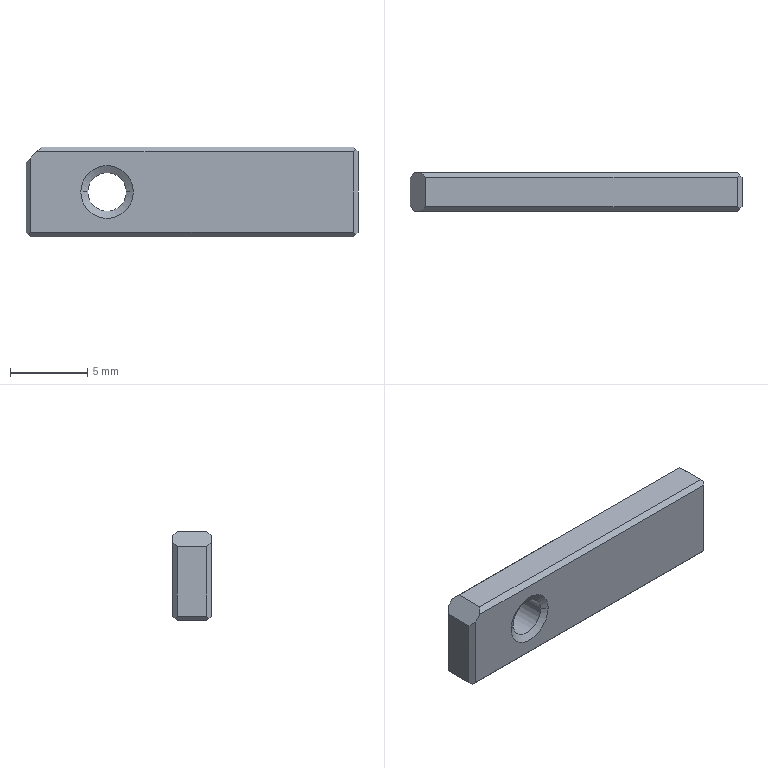Part | NX | 1 solid | 22 faces | box 21.5 x 2.5 x 5.8 mm | volume 292.746 mm3 | plane 18 | cylinder 2 | cone 2 | commonest cylinder face diameters 2.5 x2
STEP:
#1=CARTESIAN_POINT('',(-222.5,223.3,-37.742));
#2=VERTEX_POINT('',#1);
#3=CARTESIAN_POINT('',(-222.5,225.2,-37.742));
#4=VERTEX_POINT('',#3);
#5=CARTESIAN_POINT('',(-222.5,224.25,-37.742));
#6=DIRECTION('',(0.,1.,0.));
#7=VECTOR('',#6,1000.);
#8=LINE('',#5,#7);
#9=EDGE_CURVE('',#2,#4,#8,.T.);
#10=ORIENTED_EDGE('',*,*,#9,.F.);
#11=CARTESIAN_POINT('',(-202.3,223.3,-37.742));
#12=VERTEX_POINT('',#11);
#13=CARTESIAN_POINT('',(-212.75,223.3,-37.742));
#14=DIRECTION('',(-1.,0.,0.));
#15=VECTOR('',#14,1000.);
#16=LINE('',#13,#15);
#17=EDGE_CURVE('',#12,#2,#16,.T.);
#18=ORIENTED_EDGE('',*,*,#17,.F.);
#19=CARTESIAN_POINT('',(-202.3,225.2,-37.742));
#20=VERTEX_POINT('',#19);
#21=CARTESIAN_POINT('',(-202.3,224.25,-37.742));
#22=DIRECTION('',(0.,1.,0.));
#23=VECTOR('',#22,1000.);
#24=LINE('',#21,#23);
#25=EDGE_CURVE('',#12,#20,#24,.T.);
#26=ORIENTED_EDGE('',*,*,#25,.T.);
#27=CARTESIAN_POINT('',(-212.75,225.2,-37.742));
#28=DIRECTION('',(-1.,0.,0.));
#29=VECTOR('',#28,1000.);
#30=LINE('',#27,#29);
#31=EDGE_CURVE('',#20,#4,#30,.T.);
#32=ORIENTED_EDGE('',*,*,#31,.T.);
#33=EDGE_LOOP('',(#10,#18,#26,#32));
#34=FACE_BOUND('',#33,.T.);
#35=CARTESIAN_POINT('',(-213.,223.,-37.742));
#36=DIRECTION('',(0.,0.,1.));
#37=DIRECTION('',(0.,-1.,0.));
#38=AXIS2_PLACEMENT_3D('',#35,#36,#37);
#39=PLANE('',#38);
#40=ADVANCED_FACE('',(#34),#39,.T.);
#41=CARTESIAN_POINT('',(-223.5,223.3,-38.742));
#42=VERTEX_POINT('',#41);
#43=CARTESIAN_POINT('',(-223.5,223.3,-43.242));
#44=VERTEX_POINT('',#43);
#45=CARTESIAN_POINT('',(-223.5,223.3,-40.642));
#46=DIRECTION('',(0.,0.,-1.));
#47=VECTOR('',#46,1000.);
#48=LINE('',#45,#47);
#49=EDGE_CURVE('',#42,#44,#48,.T.);
#50=ORIENTED_EDGE('',*,*,#49,.F.);
#51=CARTESIAN_POINT('',(-223.5,225.2,-38.742));
#52=VERTEX_POINT('',#51);
#53=CARTESIAN_POINT('',(-223.5,224.25,-38.742));
#54=DIRECTION('',(0.,1.,0.));
#55=VECTOR('',#54,1000.);
#56=LINE('',#53,#55);
#57=EDGE_CURVE('',#42,#52,#56,.T.);
#58=ORIENTED_EDGE('',*,*,#57,.T.);
#59=CARTESIAN_POINT('',(-223.5,225.2,-43.242));
#60=VERTEX_POINT('',#59);
#61=CARTESIAN_POINT('',(-223.5,225.2,-40.642));
#62=DIRECTION('',(0.,0.,-1.));
#63=VECTOR('',#62,1000.);
#64=LINE('',#61,#63);
#65=EDGE_CURVE('',#52,#60,#64,.T.);
#66=ORIENTED_EDGE('',*,*,#65,.T.);
#67=CARTESIAN_POINT('',(-223.5,224.25,-43.242));
#68=DIRECTION('',(0.,1.,0.));
#69=VECTOR('',#68,1000.);
#70=LINE('',#67,#69);
#71=EDGE_CURVE('',#44,#60,#70,.T.);
#72=ORIENTED_EDGE('',*,*,#71,.F.);
#73=EDGE_LOOP('',(#50,#58,#66,#72));
#74=FACE_BOUND('',#73,.T.);
#75=CARTESIAN_POINT('',(-223.5,223.,-37.742));
#76=DIRECTION('',(-1.,0.,0.));
#77=DIRECTION('',(0.,1.,0.));
#78=AXIS2_PLACEMENT_3D('',#75,#76,#77);
#79=PLANE('',#78);
#80=ADVANCED_FACE('',(#74),#79,.T.);
#81=CARTESIAN_POINT('',(-223.2,223.3,-43.542));
#82=VERTEX_POINT('',#81);
#83=CARTESIAN_POINT('',(-223.2,225.2,-43.542));
#84=VERTEX_POINT('',#83);
#85=CARTESIAN_POINT('',(-223.2,224.25,-43.542));
#86=DIRECTION('',(0.,1.,0.));
#87=VECTOR('',#86,1000.);
#88=LINE('',#85,#87);
#89=EDGE_CURVE('',#82,#84,#88,.T.);
#90=ORIENTED_EDGE('',*,*,#89,.T.);
#91=CARTESIAN_POINT('',(-202.3,225.2,-43.542));
#92=VERTEX_POINT('',#91);
#93=CARTESIAN_POINT('',(-212.75,225.2,-43.542));
#94=DIRECTION('',(1.,0.,0.));
#95=VECTOR('',#94,1000.);
#96=LINE('',#93,#95);
#97=EDGE_CURVE('',#84,#92,#96,.T.);
#98=ORIENTED_EDGE('',*,*,#97,.T.);
#99=CARTESIAN_POINT('',(-202.3,223.3,-43.542));
#100=VERTEX_POINT('',#99);
#101=CARTESIAN_POINT('',(-202.3,224.25,-43.542));
#102=DIRECTION('',(0.,1.,0.));
#103=VECTOR('',#102,1000.);
#104=LINE('',#101,#103);
#105=EDGE_CURVE('',#100,#92,#104,.T.);
#106=ORIENTED_EDGE('',*,*,#105,.F.);
#107=CARTESIAN_POINT('',(-212.75,223.3,-43.542));
#108=DIRECTION('',(1.,0.,0.));
#109=VECTOR('',#108,1000.);
#110=LINE('',#107,#109);
#111=EDGE_CURVE('',#82,#100,#110,.T.);
#112=ORIENTED_EDGE('',*,*,#111,.F.);
#113=EDGE_LOOP('',(#90,#98,#106,#112));
#114=FACE_BOUND('',#113,.T.);
#115=CARTESIAN_POINT('',(-223.5,223.,-43.542));
#116=DIRECTION('',(0.,0.,-1.));
#117=DIRECTION('',(-1.,0.,0.));
#118=AXIS2_PLACEMENT_3D('',#115,#116,#117);
#119=PLANE('',#118);
#120=ADVANCED_FACE('',(#114),#119,.T.);
#121=CARTESIAN_POINT('',(-217.,223.26,-40.642));
#122=VERTEX_POINT('',#121);
#123=CARTESIAN_POINT('',(-219.5,223.26,-40.642));
#124=VERTEX_POINT('',#123);
#125=CARTESIAN_POINT('',(-218.25,223.26,-40.642));
#126=DIRECTION('',(0.,-1.,0.));
#127=DIRECTION('',(-1.,0.,0.));
#128=AXIS2_PLACEMENT_3D('',#125,#126,#127);
#129=CIRCLE('',#128,1.25);
#130=EDGE_CURVE('',#122,#124,#129,.T.);
#131=ORIENTED_EDGE('',*,*,#130,.T.);
#132=CARTESIAN_POINT('',(-219.5,225.5,-40.642));
#133=VERTEX_POINT('',#132);
#134=CARTESIAN_POINT('',(-219.5,223.,-40.642));
#135=DIRECTION('',(0.,-1.,0.));
#136=VECTOR('',#135,1000.);
#137=LINE('',#134,#136);
#138=EDGE_CURVE('',#124,#133,#137,.F.);
#139=ORIENTED_EDGE('',*,*,#138,.T.);
#140=CARTESIAN_POINT('',(-217.,225.5,-40.642));
#141=VERTEX_POINT('',#140);
#142=CARTESIAN_POINT('',(-218.25,225.5,-40.642));
#143=DIRECTION('',(0.,-1.,0.));
#144=DIRECTION('',(-1.,0.,0.));
#145=AXIS2_PLACEMENT_3D('',#142,#143,#144);
#146=CIRCLE('',#145,1.25);
#147=EDGE_CURVE('',#141,#133,#146,.T.);
#148=ORIENTED_EDGE('',*,*,#147,.F.);
#149=CARTESIAN_POINT('',(-217.,223.,-40.642));
#150=DIRECTION('',(0.,-1.,0.));
#151=VECTOR('',#150,1000.);
#152=LINE('',#149,#151);
#153=EDGE_CURVE('',#122,#141,#152,.F.);
#154=ORIENTED_EDGE('',*,*,#153,.F.);
#155=EDGE_LOOP('',(#131,#139,#148,#154));
#156=FACE_BOUND('',#155,.T.);
#157=CARTESIAN_POINT('',(-218.25,223.,-40.642));
#158=DIRECTION('',(0.,-1.,0.));
#159=DIRECTION('',(-1.,0.,0.));
#160=AXIS2_PLACEMENT_3D('',#157,#158,#159);
#161=CYLINDRICAL_SURFACE('',#160,1.25);
#162=ADVANCED_FACE('',(#156),#161,.F.);
#163=ORIENTED_EDGE('',*,*,#130,.F.);
#164=CARTESIAN_POINT('',(-216.55,223.,-40.642));
#165=VERTEX_POINT('',#164);
#166=CARTESIAN_POINT('',(-217.,223.26,-40.642));
#167=DIRECTION('',(0.866,-0.5,0.));
#168=VECTOR('',#167,1000.);
#169=LINE('',#166,#168);
#170=EDGE_CURVE('',#165,#122,#169,.F.);
#171=ORIENTED_EDGE('',*,*,#170,.F.);
#172=CARTESIAN_POINT('',(-219.95,223.,-40.642));
#173=VERTEX_POINT('',#172);
#174=CARTESIAN_POINT('',(-218.25,223.,-40.642));
#175=DIRECTION('',(0.,-1.,0.));
#176=DIRECTION('',(-1.,0.,0.));
#177=AXIS2_PLACEMENT_3D('',#174,#175,#176);
#178=CIRCLE('',#177,1.7);
#179=EDGE_CURVE('',#165,#173,#178,.T.);
#180=ORIENTED_EDGE('',*,*,#179,.T.);
#181=CARTESIAN_POINT('',(-219.5,223.26,-40.642));
#182=DIRECTION('',(-0.866,-0.5,0.));
#183=VECTOR('',#182,1000.);
#184=LINE('',#181,#183);
#185=EDGE_CURVE('',#173,#124,#184,.F.);
#186=ORIENTED_EDGE('',*,*,#185,.T.);
#187=EDGE_LOOP('',(#163,#171,#180,#186));
#188=FACE_BOUND('',#187,.T.);
#189=CARTESIAN_POINT('',(-218.25,223.26,-40.642));
#190=DIRECTION('',(0.,-1.,0.));
#191=DIRECTION('',(-1.,0.,0.));
#192=AXIS2_PLACEMENT_3D('',#189,#190,#191);
#193=CONICAL_SURFACE('',#192,1.25,1.047);
#194=ADVANCED_FACE('',(#188),#193,.F.);
#195=ORIENTED_EDGE('',*,*,#97,.F.);
#196=CARTESIAN_POINT('',(-223.35,225.35,-43.392));
#197=VERTEX_POINT('',#196);
#198=CARTESIAN_POINT('',(-221.,223.,-45.742));
#199=DIRECTION('',(-0.5774,0.5774,0.5774));
#200=VECTOR('',#199,1000.);
#201=LINE('',#198,#200);
#202=EDGE_CURVE('',#84,#197,#201,.T.);
#203=ORIENTED_EDGE('',*,*,#202,.T.);
#204=CARTESIAN_POINT('',(-223.2,225.5,-43.242));
#205=VERTEX_POINT('',#204);
#206=CARTESIAN_POINT('',(-225.7,223.,-45.742));
#207=DIRECTION('',(-0.5774,-0.5774,-0.5774));
#208=VECTOR('',#207,1000.);
#209=LINE('',#206,#208);
#210=EDGE_CURVE('',#205,#197,#209,.T.);
#211=ORIENTED_EDGE('',*,*,#210,.F.);
#212=CARTESIAN_POINT('',(-202.3,225.5,-43.242));
#213=VERTEX_POINT('',#212);
#214=CARTESIAN_POINT('',(-212.75,225.5,-43.242));
#215=DIRECTION('',(1.,0.,0.));
#216=VECTOR('',#215,1000.);
#217=LINE('',#214,#216);
#218=EDGE_CURVE('',#205,#213,#217,.T.);
#219=ORIENTED_EDGE('',*,*,#218,.T.);
#220=CARTESIAN_POINT('',(-202.15,225.35,-43.392));
#221=VERTEX_POINT('',#220);
#222=CARTESIAN_POINT('',(-218.25,241.45,-27.292));
#223=DIRECTION('',(-0.5774,0.5774,0.5774));
#224=VECTOR('',#223,1000.);
#225=LINE('',#222,#224);
#226=EDGE_CURVE('',#221,#213,#225,.T.);
#227=ORIENTED_EDGE('',*,*,#226,.F.);
#228=CARTESIAN_POINT('',(-218.25,209.25,-59.492));
#229=DIRECTION('',(0.5774,0.5774,0.5774));
#230=VECTOR('',#229,1000.);
#231=LINE('',#228,#230);
#232=EDGE_CURVE('',#92,#221,#231,.T.);
#233=ORIENTED_EDGE('',*,*,#232,.F.);
#234=EDGE_LOOP('',(#195,#203,#211,#219,#227,#233));
#235=FACE_BOUND('',#234,.T.);
#236=CARTESIAN_POINT('',(-212.75,225.35,-43.392));
#237=DIRECTION('',(0.,0.7071,-0.7071));
#238=DIRECTION('',(-1.,0.,0.));
#239=AXIS2_PLACEMENT_3D('',#236,#237,#238);
#240=PLANE('',#239);
#241=ADVANCED_FACE('',(#235),#240,.T.);
#242=ORIENTED_EDGE('',*,*,#89,.F.);
#243=CARTESIAN_POINT('',(-223.35,223.15,-43.392));
#244=VERTEX_POINT('',#243);
#245=CARTESIAN_POINT('',(-223.5,223.,-43.242));
#246=DIRECTION('',(0.5774,0.5774,-0.5774));
#247=VECTOR('',#246,1000.);
#248=LINE('',#245,#247);
#249=EDGE_CURVE('',#244,#82,#248,.T.);
#250=ORIENTED_EDGE('',*,*,#249,.F.);
#251=CARTESIAN_POINT('',(-226.1,225.9,-40.642));
#252=DIRECTION('',(-0.5774,0.5774,0.5774));
#253=VECTOR('',#252,1000.);
#254=LINE('',#251,#253);
#255=EDGE_CURVE('',#244,#44,#254,.T.);
#256=ORIENTED_EDGE('',*,*,#255,.T.);
#257=ORIENTED_EDGE('',*,*,#71,.T.);
#258=CARTESIAN_POINT('',(-226.1,222.6,-40.642));
#259=DIRECTION('',(-0.5774,-0.5774,0.5774));
#260=VECTOR('',#259,1000.);
#261=LINE('',#258,#260);
#262=EDGE_CURVE('',#197,#60,#261,.T.);
#263=ORIENTED_EDGE('',*,*,#262,.F.);
#264=ORIENTED_EDGE('',*,*,#202,.F.);
#265=EDGE_LOOP('',(#242,#250,#256,#257,#263,#264));
#266=FACE_BOUND('',#265,.T.);
#267=CARTESIAN_POINT('',(-223.35,224.25,-43.392));
#268=DIRECTION('',(-0.7071,0.,-0.7071));
#269=DIRECTION('',(-0.7071,0.,0.7071));
#270=AXIS2_PLACEMENT_3D('',#267,#268,#269);
#271=PLANE('',#270);
#272=ADVANCED_FACE('',(#266),#271,.T.);
#273=ORIENTED_EDGE('',*,*,#9,.T.);
#274=CARTESIAN_POINT('',(-222.8,225.5,-38.042));
#275=VERTEX_POINT('',#274);
#276=CARTESIAN_POINT('',(-220.3,223.,-35.542));
#277=DIRECTION('',(-0.5774,0.5774,-0.5774));
#278=VECTOR('',#277,1000.);
#279=LINE('',#276,#278);
#280=EDGE_CURVE('',#4,#275,#279,.T.);
#281=ORIENTED_EDGE('',*,*,#280,.T.);
#282=CARTESIAN_POINT('',(-223.2,225.5,-38.442));
#283=VERTEX_POINT('',#282);
#284=CARTESIAN_POINT('',(-225.4,225.5,-40.642));
#285=DIRECTION('',(0.7071,0.,0.7071));
#286=VECTOR('',#285,1000.);
#287=LINE('',#284,#286);
#288=EDGE_CURVE('',#283,#275,#287,.T.);
#289=ORIENTED_EDGE('',*,*,#288,.F.);
#290=CARTESIAN_POINT('',(-225.7,223.,-40.942));
#291=DIRECTION('',(-0.5774,-0.5774,-0.5774));
#292=VECTOR('',#291,1000.);
#293=LINE('',#290,#292);
#294=EDGE_CURVE('',#283,#52,#293,.T.);
#295=ORIENTED_EDGE('',*,*,#294,.T.);
#296=ORIENTED_EDGE('',*,*,#57,.F.);
#297=CARTESIAN_POINT('',(-223.2,223.,-38.442));
#298=VERTEX_POINT('',#297);
#299=CARTESIAN_POINT('',(-223.2,223.,-38.442));
#300=DIRECTION('',(-0.5774,0.5774,-0.5774));
#301=VECTOR('',#300,1000.);
#302=LINE('',#299,#301);
#303=EDGE_CURVE('',#298,#42,#302,.T.);
#304=ORIENTED_EDGE('',*,*,#303,.F.);
#305=CARTESIAN_POINT('',(-222.8,223.,-38.042));
#306=VERTEX_POINT('',#305);
#307=CARTESIAN_POINT('',(-225.4,223.,-40.642));
#308=DIRECTION('',(0.7071,0.,0.7071));
#309=VECTOR('',#308,1000.);
#310=LINE('',#307,#309);
#311=EDGE_CURVE('',#298,#306,#310,.T.);
#312=ORIENTED_EDGE('',*,*,#311,.T.);
#313=CARTESIAN_POINT('',(-222.8,223.,-38.042));
#314=DIRECTION('',(-0.5774,-0.5774,-0.5774));
#315=VECTOR('',#314,1000.);
#316=LINE('',#313,#315);
#317=EDGE_CURVE('',#2,#306,#316,.T.);
#318=ORIENTED_EDGE('',*,*,#317,.F.);
#319=EDGE_LOOP('',(#273,#281,#289,#295,#296,#304,#312,#318));
#320=FACE_BOUND('',#319,.T.);
#321=CARTESIAN_POINT('',(-223.,224.25,-38.242));
#322=DIRECTION('',(0.7071,0.,-0.7071));
#323=DIRECTION('',(0.,-1.,0.));
#324=AXIS2_PLACEMENT_3D('',#321,#322,#323);
#325=PLANE('',#324);
#326=ADVANCED_FACE('',(#320),#325,.F.);
#327=ORIENTED_EDGE('',*,*,#138,.F.);
#328=CARTESIAN_POINT('',(-218.25,223.26,-40.642));
#329=DIRECTION('',(0.,-1.,0.));
#330=DIRECTION('',(-1.,0.,0.));
#331=AXIS2_PLACEMENT_3D('',#328,#329,#330);
#332=CIRCLE('',#331,1.25);
#333=EDGE_CURVE('',#124,#122,#332,.T.);
#334=ORIENTED_EDGE('',*,*,#333,.T.);
#335=ORIENTED_EDGE('',*,*,#153,.T.);
#336=CARTESIAN_POINT('',(-218.25,225.5,-40.642));
#337=DIRECTION('',(0.,-1.,0.));
#338=DIRECTION('',(-1.,0.,0.));
#339=AXIS2_PLACEMENT_3D('',#336,#337,#338);
#340=CIRCLE('',#339,1.25);
#341=EDGE_CURVE('',#133,#141,#340,.T.);
#342=ORIENTED_EDGE('',*,*,#341,.F.);
#343=EDGE_LOOP('',(#327,#334,#335,#342));
#344=FACE_BOUND('',#343,.T.);
#345=CARTESIAN_POINT('',(-218.25,223.,-40.642));
#346=DIRECTION('',(0.,-1.,0.));
#347=DIRECTION('',(-1.,0.,0.));
#348=AXIS2_PLACEMENT_3D('',#345,#346,#347);
#349=CYLINDRICAL_SURFACE('',#348,1.25);
#350=ADVANCED_FACE('',(#344),#349,.F.);
#351=ORIENTED_EDGE('',*,*,#185,.F.);
#352=CARTESIAN_POINT('',(-218.25,223.,-40.642));
#353=DIRECTION('',(0.,-1.,0.));
#354=DIRECTION('',(-1.,0.,0.));
#355=AXIS2_PLACEMENT_3D('',#352,#353,#354);
#356=CIRCLE('',#355,1.7);
#357=EDGE_CURVE('',#173,#165,#356,.T.);
#358=ORIENTED_EDGE('',*,*,#357,.T.);
#359=ORIENTED_EDGE('',*,*,#170,.T.);
#360=ORIENTED_EDGE('',*,*,#333,.F.);
#361=EDGE_LOOP('',(#351,#358,#359,#360));
#362=FACE_BOUND('',#361,.T.);
#363=CARTESIAN_POINT('',(-218.25,223.26,-40.642));
#364=DIRECTION('',(0.,-1.,0.));
#365=DIRECTION('',(-1.,0.,0.));
#366=AXIS2_PLACEMENT_3D('',#363,#364,#365);
#367=CONICAL_SURFACE('',#366,1.25,1.047);
#368=ADVANCED_FACE('',(#362),#367,.F.);
#369=CARTESIAN_POINT('',(-223.2,225.5,-40.642));
#370=DIRECTION('',(0.,0.,-1.));
#371=VECTOR('',#370,1000.);
#372=LINE('',#369,#371);
#373=EDGE_CURVE('',#283,#205,#372,.T.);
#374=ORIENTED_EDGE('',*,*,#373,.F.);
#375=ORIENTED_EDGE('',*,*,#288,.T.);
#376=CARTESIAN_POINT('',(-202.3,225.5,-38.042));
#377=VERTEX_POINT('',#376);
#378=CARTESIAN_POINT('',(-212.75,225.5,-38.042));
#379=DIRECTION('',(-1.,0.,0.));
#380=VECTOR('',#379,1000.);
#381=LINE('',#378,#380);
#382=EDGE_CURVE('',#377,#275,#381,.T.);
#383=ORIENTED_EDGE('',*,*,#382,.F.);
#384=CARTESIAN_POINT('',(-202.3,225.5,-40.642));
#385=DIRECTION('',(0.,0.,1.));
#386=VECTOR('',#385,1000.);
#387=LINE('',#384,#386);
#388=EDGE_CURVE('',#213,#377,#387,.T.);
#389=ORIENTED_EDGE('',*,*,#388,.F.);
#390=ORIENTED_EDGE('',*,*,#218,.F.);
#391=EDGE_LOOP('',(#374,#375,#383,#389,#390));
#392=FACE_BOUND('',#391,.T.);
#393=ORIENTED_EDGE('',*,*,#147,.T.);
#394=ORIENTED_EDGE('',*,*,#341,.T.);
#395=EDGE_LOOP('',(#393,#394));
#396=FACE_BOUND('',#395,.T.);
#397=CARTESIAN_POINT('',(-218.25,225.5,-40.642));
#398=DIRECTION('',(0.,1.,0.));
#399=DIRECTION('',(0.,0.,-1.));
#400=AXIS2_PLACEMENT_3D('',#397,#398,#399);
#401=PLANE('',#400);
#402=ADVANCED_FACE('',(#392,#396),#401,.T.);
#403=ORIENTED_EDGE('',*,*,#382,.T.);
#404=ORIENTED_EDGE('',*,*,#280,.F.);
#405=ORIENTED_EDGE('',*,*,#31,.F.);
#406=CARTESIAN_POINT('',(-202.15,225.35,-37.892));
#407=VERTEX_POINT('',#406);
#408=CARTESIAN_POINT('',(-218.25,209.25,-21.792));
#409=DIRECTION('',(0.5774,0.5774,-0.5774));
#410=VECTOR('',#409,1000.);
#411=LINE('',#408,#410);
#412=EDGE_CURVE('',#20,#407,#411,.T.);
#413=ORIENTED_EDGE('',*,*,#412,.T.);
#414=CARTESIAN_POINT('',(-218.25,241.45,-53.992));
#415=DIRECTION('',(-0.5774,0.5774,-0.5774));
#416=VECTOR('',#415,1000.);
#417=LINE('',#414,#416);
#418=EDGE_CURVE('',#407,#377,#417,.T.);
#419=ORIENTED_EDGE('',*,*,#418,.T.);
#420=EDGE_LOOP('',(#403,#404,#405,#413,#419));
#421=FACE_BOUND('',#420,.T.);
#422=CARTESIAN_POINT('',(-212.75,225.35,-37.892));
#423=DIRECTION('',(0.,-0.7071,-0.7071));
#424=DIRECTION('',(0.,-0.7071,0.7071));
#425=AXIS2_PLACEMENT_3D('',#422,#423,#424);
#426=PLANE('',#425);
#427=ADVANCED_FACE('',(#421),#426,.F.);
#428=ORIENTED_EDGE('',*,*,#373,.T.);
#429=ORIENTED_EDGE('',*,*,#210,.T.);
#430=ORIENTED_EDGE('',*,*,#262,.T.);
#431=ORIENTED_EDGE('',*,*,#65,.F.);
#432=ORIENTED_EDGE('',*,*,#294,.F.);
#433=EDGE_LOOP('',(#428,#429,#430,#431,#432));
#434=FACE_BOUND('',#433,.T.);
#435=CARTESIAN_POINT('',(-223.35,225.35,-40.642));
#436=DIRECTION('',(0.7071,-0.7071,0.));
#437=DIRECTION('',(0.,0.,-1.));
#438=AXIS2_PLACEMENT_3D('',#435,#436,#437);
#439=PLANE('',#438);
#440=ADVANCED_FACE('',(#434),#439,.F.);
#441=CARTESIAN_POINT('',(-202.,223.3,-43.242));
#442=VERTEX_POINT('',#441);
#443=CARTESIAN_POINT('',(-202.,225.2,-43.242));
#444=VERTEX_POINT('',#443);
#445=CARTESIAN_POINT('',(-202.,224.25,-43.242));
#446=DIRECTION('',(0.,1.,0.));
#447=VECTOR('',#446,1000.);
#448=LINE('',#445,#447);
#449=EDGE_CURVE('',#442,#444,#448,.T.);
#450=ORIENTED_EDGE('',*,*,#449,.T.);
#451=CARTESIAN_POINT('',(-202.,225.2,-38.042));
#452=VERTEX_POINT('',#451);
#453=CARTESIAN_POINT('',(-202.,225.2,-40.642));
#454=DIRECTION('',(0.,0.,1.));
#455=VECTOR('',#454,1000.);
#456=LINE('',#453,#455);
#457=EDGE_CURVE('',#444,#452,#456,.T.);
#458=ORIENTED_EDGE('',*,*,#457,.T.);
#459=CARTESIAN_POINT('',(-202.,223.3,-38.042));
#460=VERTEX_POINT('',#459);
#461=CARTESIAN_POINT('',(-202.,224.25,-38.042));
#462=DIRECTION('',(0.,1.,0.));
#463=VECTOR('',#462,1000.);
#464=LINE('',#461,#463);
#465=EDGE_CURVE('',#460,#452,#464,.T.);
#466=ORIENTED_EDGE('',*,*,#465,.F.);
#467=CARTESIAN_POINT('',(-202.,223.3,-40.642));
#468=DIRECTION('',(0.,0.,1.));
#469=VECTOR('',#468,1000.);
#470=LINE('',#467,#469);
#471=EDGE_CURVE('',#442,#460,#470,.T.);
#472=ORIENTED_EDGE('',*,*,#471,.F.);
#473=EDGE_LOOP('',(#450,#458,#466,#472));
#474=FACE_BOUND('',#473,.T.);
#475=CARTESIAN_POINT('',(-202.,223.,-43.542));
#476=DIRECTION('',(1.,0.,0.));
#477=DIRECTION('',(0.,1.,0.));
#478=AXIS2_PLACEMENT_3D('',#475,#476,#477);
#479=PLANE('',#478);
#480=ADVANCED_FACE('',(#474),#479,.T.);
#481=ORIENTED_EDGE('',*,*,#457,.F.);
#482=CARTESIAN_POINT('',(-218.25,241.45,-59.492));
#483=DIRECTION('',(-0.5774,0.5774,-0.5774));
#484=VECTOR('',#483,1000.);
#485=LINE('',#482,#484);
#486=EDGE_CURVE('',#444,#221,#485,.T.);
#487=ORIENTED_EDGE('',*,*,#486,.T.);
#488=ORIENTED_EDGE('',*,*,#226,.T.);
#489=ORIENTED_EDGE('',*,*,#388,.T.);
#490=ORIENTED_EDGE('',*,*,#418,.F.);
#491=CARTESIAN_POINT('',(-218.25,241.45,-21.792));
#492=DIRECTION('',(-0.5774,0.5774,0.5774));
#493=VECTOR('',#492,1000.);
#494=LINE('',#491,#493);
#495=EDGE_CURVE('',#452,#407,#494,.T.);
#496=ORIENTED_EDGE('',*,*,#495,.F.);
#497=EDGE_LOOP('',(#481,#487,#488,#489,#490,#496));
#498=FACE_BOUND('',#497,.T.);
#499=CARTESIAN_POINT('',(-202.15,225.35,-40.642));
#500=DIRECTION('',(0.7071,0.7071,0.));
#501=DIRECTION('',(0.,0.,-1.));
#502=AXIS2_PLACEMENT_3D('',#499,#500,#501);
#503=PLANE('',#502);
#504=ADVANCED_FACE('',(#498),#503,.T.);
#505=ORIENTED_EDGE('',*,*,#465,.T.);
#506=ORIENTED_EDGE('',*,*,#495,.T.);
#507=ORIENTED_EDGE('',*,*,#412,.F.);
#508=ORIENTED_EDGE('',*,*,#25,.F.);
#509=CARTESIAN_POINT('',(-202.15,223.15,-37.892));
#510=VERTEX_POINT('',#509);
#511=CARTESIAN_POINT('',(-218.25,239.25,-21.792));
#512=DIRECTION('',(0.5774,-0.5774,-0.5774));
#513=VECTOR('',#512,1000.);
#514=LINE('',#511,#513);
#515=EDGE_CURVE('',#12,#510,#514,.T.);
#516=ORIENTED_EDGE('',*,*,#515,.T.);
#517=CARTESIAN_POINT('',(-218.25,207.05,-21.792));
#518=DIRECTION('',(0.5774,0.5774,-0.5774));
#519=VECTOR('',#518,1000.);
#520=LINE('',#517,#519);
#521=EDGE_CURVE('',#510,#460,#520,.T.);
#522=ORIENTED_EDGE('',*,*,#521,.T.);
#523=EDGE_LOOP('',(#505,#506,#507,#508,#516,#522));
#524=FACE_BOUND('',#523,.T.);
#525=CARTESIAN_POINT('',(-202.15,224.25,-37.892));
#526=DIRECTION('',(-0.7071,0.,-0.7071));
#527=DIRECTION('',(-0.7071,0.,0.7071));
#528=AXIS2_PLACEMENT_3D('',#525,#526,#527);
#529=PLANE('',#528);
#530=ADVANCED_FACE('',(#524),#529,.F.);
#531=ORIENTED_EDGE('',*,*,#471,.T.);
#532=ORIENTED_EDGE('',*,*,#521,.F.);
#533=CARTESIAN_POINT('',(-202.3,223.,-38.042));
#534=VERTEX_POINT('',#533);
#535=CARTESIAN_POINT('',(-218.25,207.05,-53.992));
#536=DIRECTION('',(-0.5774,-0.5774,-0.5774));
#537=VECTOR('',#536,1000.);
#538=LINE('',#535,#537);
#539=EDGE_CURVE('',#510,#534,#538,.T.);
#540=ORIENTED_EDGE('',*,*,#539,.T.);
#541=CARTESIAN_POINT('',(-202.3,223.,-43.242));
#542=VERTEX_POINT('',#541);
#543=CARTESIAN_POINT('',(-202.3,223.,-40.642));
#544=DIRECTION('',(0.,0.,1.));
#545=VECTOR('',#544,1000.);
#546=LINE('',#543,#545);
#547=EDGE_CURVE('',#542,#534,#546,.T.);
#548=ORIENTED_EDGE('',*,*,#547,.F.);
#549=CARTESIAN_POINT('',(-202.15,223.15,-43.392));
#550=VERTEX_POINT('',#549);
#551=CARTESIAN_POINT('',(-218.25,207.05,-27.292));
#552=DIRECTION('',(-0.5774,-0.5774,0.5774));
#553=VECTOR('',#552,1000.);
#554=LINE('',#551,#553);
#555=EDGE_CURVE('',#550,#542,#554,.T.);
#556=ORIENTED_EDGE('',*,*,#555,.F.);
#557=CARTESIAN_POINT('',(-218.25,207.05,-59.492));
#558=DIRECTION('',(-0.5774,-0.5774,-0.5774));
#559=VECTOR('',#558,1000.);
#560=LINE('',#557,#559);
#561=EDGE_CURVE('',#442,#550,#560,.T.);
#562=ORIENTED_EDGE('',*,*,#561,.F.);
#563=EDGE_LOOP('',(#531,#532,#540,#548,#556,#562));
#564=FACE_BOUND('',#563,.T.);
#565=CARTESIAN_POINT('',(-202.15,223.15,-40.642));
#566=DIRECTION('',(-0.7071,0.7071,0.));
#567=DIRECTION('',(0.,0.,1.));
#568=AXIS2_PLACEMENT_3D('',#565,#566,#567);
#569=PLANE('',#568);
#570=ADVANCED_FACE('',(#564),#569,.F.);
#571=ORIENTED_EDGE('',*,*,#449,.F.);
#572=ORIENTED_EDGE('',*,*,#561,.T.);
#573=CARTESIAN_POINT('',(-218.25,239.25,-59.492));
#574=DIRECTION('',(-0.5774,0.5774,-0.5774));
#575=VECTOR('',#574,1000.);
#576=LINE('',#573,#575);
#577=EDGE_CURVE('',#550,#100,#576,.T.);
#578=ORIENTED_EDGE('',*,*,#577,.T.);
#579=ORIENTED_EDGE('',*,*,#105,.T.);
#580=ORIENTED_EDGE('',*,*,#232,.T.);
#581=ORIENTED_EDGE('',*,*,#486,.F.);
#582=EDGE_LOOP('',(#571,#572,#578,#579,#580,#581));
#583=FACE_BOUND('',#582,.T.);
#584=CARTESIAN_POINT('',(-202.15,224.25,-43.392));
#585=DIRECTION('',(0.7071,0.,-0.7071));
#586=DIRECTION('',(0.,-1.,0.));
#587=AXIS2_PLACEMENT_3D('',#584,#585,#586);
#588=PLANE('',#587);
#589=ADVANCED_FACE('',(#583),#588,.T.);
#590=CARTESIAN_POINT('',(-223.2,223.,-43.242));
#591=VERTEX_POINT('',#590);
#592=CARTESIAN_POINT('',(-223.2,223.,-40.642));
#593=DIRECTION('',(0.,0.,-1.));
#594=VECTOR('',#593,1000.);
#595=LINE('',#592,#594);
#596=EDGE_CURVE('',#298,#591,#595,.T.);
#597=ORIENTED_EDGE('',*,*,#596,.T.);
#598=CARTESIAN_POINT('',(-212.75,223.,-43.242));
#599=DIRECTION('',(1.,0.,0.));
#600=VECTOR('',#599,1000.);
#601=LINE('',#598,#600);
#602=EDGE_CURVE('',#591,#542,#601,.T.);
#603=ORIENTED_EDGE('',*,*,#602,.T.);
#604=ORIENTED_EDGE('',*,*,#547,.T.);
#605=CARTESIAN_POINT('',(-212.75,223.,-38.042));
#606=DIRECTION('',(-1.,0.,0.));
#607=VECTOR('',#606,1000.);
#608=LINE('',#605,#607);
#609=EDGE_CURVE('',#534,#306,#608,.T.);
#610=ORIENTED_EDGE('',*,*,#609,.T.);
#611=ORIENTED_EDGE('',*,*,#311,.F.);
#612=EDGE_LOOP('',(#597,#603,#604,#610,#611));
#613=FACE_BOUND('',#612,.T.);
#614=ORIENTED_EDGE('',*,*,#179,.F.);
#615=ORIENTED_EDGE('',*,*,#357,.F.);
#616=EDGE_LOOP('',(#614,#615));
#617=FACE_BOUND('',#616,.T.);
#618=CARTESIAN_POINT('',(-218.25,223.,-40.642));
#619=DIRECTION('',(0.,1.,0.));
#620=DIRECTION('',(0.,0.,-1.));
#621=AXIS2_PLACEMENT_3D('',#618,#619,#620);
#622=PLANE('',#621);
#623=ADVANCED_FACE('',(#613,#617),#622,.F.);
#624=ORIENTED_EDGE('',*,*,#609,.F.);
#625=ORIENTED_EDGE('',*,*,#539,.F.);
#626=ORIENTED_EDGE('',*,*,#515,.F.);
#627=ORIENTED_EDGE('',*,*,#17,.T.);
#628=ORIENTED_EDGE('',*,*,#317,.T.);
#629=EDGE_LOOP('',(#624,#625,#626,#627,#628));
#630=FACE_BOUND('',#629,.T.);
#631=CARTESIAN_POINT('',(-212.75,223.15,-37.892));
#632=DIRECTION('',(0.,-0.7071,0.7071));
#633=DIRECTION('',(-1.,0.,0.));
#634=AXIS2_PLACEMENT_3D('',#631,#632,#633);
#635=PLANE('',#634);
#636=ADVANCED_FACE('',(#630),#635,.T.);
#637=ORIENTED_EDGE('',*,*,#602,.F.);
#638=CARTESIAN_POINT('',(-223.2,223.,-43.242));
#639=DIRECTION('',(-0.5774,0.5774,-0.5774));
#640=VECTOR('',#639,1000.);
#641=LINE('',#638,#640);
#642=EDGE_CURVE('',#591,#244,#641,.T.);
#643=ORIENTED_EDGE('',*,*,#642,.T.);
#644=ORIENTED_EDGE('',*,*,#249,.T.);
#645=ORIENTED_EDGE('',*,*,#111,.T.);
#646=ORIENTED_EDGE('',*,*,#577,.F.);
#647=ORIENTED_EDGE('',*,*,#555,.T.);
#648=EDGE_LOOP('',(#637,#643,#644,#645,#646,#647));
#649=FACE_BOUND('',#648,.T.);
#650=CARTESIAN_POINT('',(-212.75,223.15,-43.392));
#651=DIRECTION('',(0.,-0.7071,-0.7071));
#652=DIRECTION('',(0.,-0.7071,0.7071));
#653=AXIS2_PLACEMENT_3D('',#650,#651,#652);
#654=PLANE('',#653);
#655=ADVANCED_FACE('',(#649),#654,.T.);
#656=ORIENTED_EDGE('',*,*,#596,.F.);
#657=ORIENTED_EDGE('',*,*,#303,.T.);
#658=ORIENTED_EDGE('',*,*,#49,.T.);
#659=ORIENTED_EDGE('',*,*,#255,.F.);
#660=ORIENTED_EDGE('',*,*,#642,.F.);
#661=EDGE_LOOP('',(#656,#657,#658,#659,#660));
#662=FACE_BOUND('',#661,.T.);
#663=CARTESIAN_POINT('',(-223.35,223.15,-40.642));
#664=DIRECTION('',(-0.7071,-0.7071,0.));
#665=DIRECTION('',(-0.7071,0.7071,0.));
#666=AXIS2_PLACEMENT_3D('',#663,#664,#665);
#667=PLANE('',#666);
#668=ADVANCED_FACE('',(#662),#667,.T.);
#669=CLOSED_SHELL('',(#40,#80,#120,#162,#194,#241,#272,#326,#350,#368,#402,#427,#440,#480,#504,#530,#570,#589,#623,#636,#655,#668));
#670=MANIFOLD_SOLID_BREP('',#669);
#671=(LENGTH_UNIT()NAMED_UNIT(*)SI_UNIT(.MILLI.,.METRE.));
#672=UNCERTAINTY_MEASURE_WITH_UNIT(LENGTH_MEASURE(0.00001),#671,'','');
#673=(NAMED_UNIT(*)PLANE_ANGLE_UNIT()SI_UNIT($,.RADIAN.));
#674=(NAMED_UNIT(*)SI_UNIT($,.STERADIAN.)SOLID_ANGLE_UNIT());
#675=(GEOMETRIC_REPRESENTATION_CONTEXT(3)GLOBAL_UNCERTAINTY_ASSIGNED_CONTEXT((#672))GLOBAL_UNIT_ASSIGNED_CONTEXT((#671,#673,#674))REPRESENTATION_CONTEXT('',''));
#676=ADVANCED_BREP_SHAPE_REPRESENTATION('',(#670),#675);